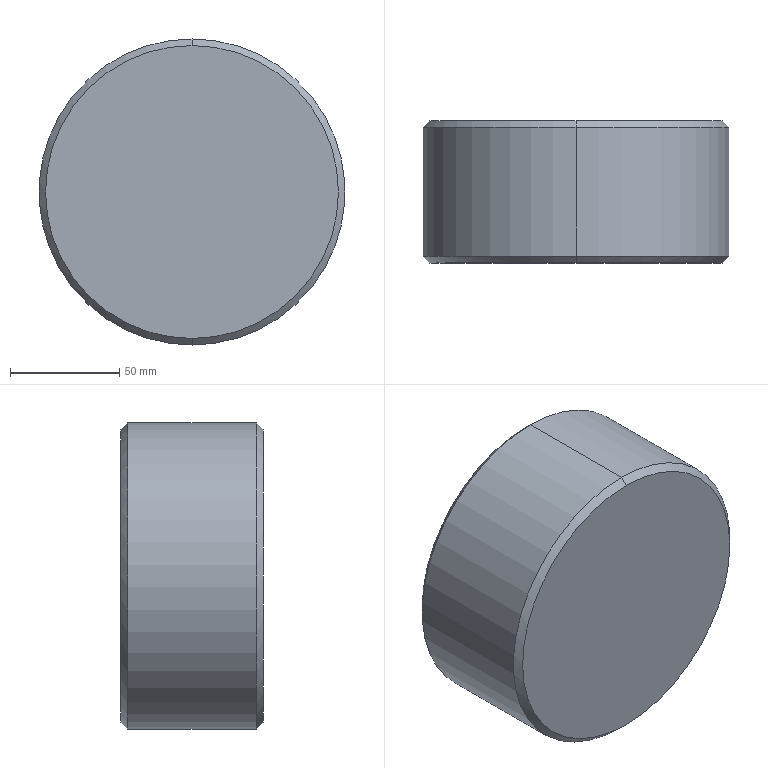Part | SolidWorks | features BaseBody 1 | 1 solid | 13 faces | box 140 x 65 x 140 mm | volume 687379 mm3 | cone 4 | cylinder 4 | plane 3 | sphere 2 | commonest cylinder face diameters 110 x2 140 x2
STEP:
#1=CARTESIAN_POINT('',(234.677,585.635,330.107));
#2=VERTEX_POINT('',#1);
#3=CARTESIAN_POINT('',(234.677,588.635,327.107));
#4=VERTEX_POINT('',#3);
#5=CARTESIAN_POINT('',(234.677,588.635,327.107));
#6=DIRECTION('',(0.,0.7071,-0.7071));
#7=VECTOR('',#6,1000.);
#8=LINE('',#5,#7);
#9=EDGE_CURVE('',#2,#4,#8,.T.);
#10=ORIENTED_EDGE('',*,*,#9,.T.);
#11=CARTESIAN_POINT('',(234.677,588.635,193.107));
#12=VERTEX_POINT('',#11);
#13=CARTESIAN_POINT('',(234.677,588.635,260.107));
#14=DIRECTION('',(0.,1.,0.));
#15=DIRECTION('',(0.,0.,1.));
#16=AXIS2_PLACEMENT_3D('',#13,#14,#15);
#17=CIRCLE('',#16,67.);
#18=EDGE_CURVE('',#12,#4,#17,.T.);
#19=ORIENTED_EDGE('',*,*,#18,.F.);
#20=CARTESIAN_POINT('',(234.677,585.635,190.107));
#21=VERTEX_POINT('',#20);
#22=CARTESIAN_POINT('',(234.677,588.635,193.107));
#23=DIRECTION('',(0.,0.7071,0.7071));
#24=VECTOR('',#23,1000.);
#25=LINE('',#22,#24);
#26=EDGE_CURVE('',#21,#12,#25,.T.);
#27=ORIENTED_EDGE('',*,*,#26,.F.);
#28=CARTESIAN_POINT('',(234.677,585.635,260.107));
#29=DIRECTION('',(0.,-1.,0.));
#30=DIRECTION('',(0.,0.,1.));
#31=AXIS2_PLACEMENT_3D('',#28,#29,#30);
#32=CIRCLE('',#31,70.);
#33=EDGE_CURVE('',#2,#21,#32,.T.);
#34=ORIENTED_EDGE('',*,*,#33,.F.);
#35=EDGE_LOOP('',(#10,#19,#27,#34));
#36=FACE_OUTER_BOUND('',#35,.T.);
#37=CARTESIAN_POINT('',(234.677,588.635,260.107));
#38=DIRECTION('',(0.,-1.,0.));
#39=DIRECTION('',(0.,0.,1.));
#40=AXIS2_PLACEMENT_3D('',#37,#38,#39);
#41=CONICAL_SURFACE('',#40,67.,0.7854);
#42=ADVANCED_FACE('',(#36),#41,.T.);
#43=CARTESIAN_POINT('',(234.677,526.635,190.107));
#44=VERTEX_POINT('',#43);
#45=CARTESIAN_POINT('',(234.677,523.635,193.107));
#46=VERTEX_POINT('',#45);
#47=CARTESIAN_POINT('',(234.677,523.635,193.107));
#48=DIRECTION('',(0.,-0.7071,0.7071));
#49=VECTOR('',#48,1000.);
#50=LINE('',#47,#49);
#51=EDGE_CURVE('',#44,#46,#50,.T.);
#52=ORIENTED_EDGE('',*,*,#51,.T.);
#53=CARTESIAN_POINT('',(234.677,523.635,327.107));
#54=VERTEX_POINT('',#53);
#55=CARTESIAN_POINT('',(234.677,523.635,260.107));
#56=DIRECTION('',(0.,-1.,0.));
#57=DIRECTION('',(0.,0.,1.));
#58=AXIS2_PLACEMENT_3D('',#55,#56,#57);
#59=CIRCLE('',#58,67.);
#60=EDGE_CURVE('',#54,#46,#59,.T.);
#61=ORIENTED_EDGE('',*,*,#60,.F.);
#62=CARTESIAN_POINT('',(234.677,526.635,330.107));
#63=VERTEX_POINT('',#62);
#64=CARTESIAN_POINT('',(234.677,523.635,327.107));
#65=DIRECTION('',(0.,-0.7071,-0.7071));
#66=VECTOR('',#65,1000.);
#67=LINE('',#64,#66);
#68=EDGE_CURVE('',#63,#54,#67,.T.);
#69=ORIENTED_EDGE('',*,*,#68,.F.);
#70=CARTESIAN_POINT('',(234.677,526.635,260.107));
#71=DIRECTION('',(0.,1.,0.));
#72=DIRECTION('',(0.,0.,1.));
#73=AXIS2_PLACEMENT_3D('',#70,#71,#72);
#74=CIRCLE('',#73,70.);
#75=EDGE_CURVE('',#44,#63,#74,.T.);
#76=ORIENTED_EDGE('',*,*,#75,.F.);
#77=EDGE_LOOP('',(#52,#61,#69,#76));
#78=FACE_OUTER_BOUND('',#77,.T.);
#79=CARTESIAN_POINT('',(234.677,523.635,260.107));
#80=DIRECTION('',(0.,1.,0.));
#81=DIRECTION('',(0.,0.,-1.));
#82=AXIS2_PLACEMENT_3D('',#79,#80,#81);
#83=CONICAL_SURFACE('',#82,67.,0.7854);
#84=ADVANCED_FACE('',(#78),#83,.T.);
#85=CARTESIAN_POINT('',(234.677,523.635,330.107));
#86=DIRECTION('',(0.,1.,0.));
#87=VECTOR('',#86,1000.);
#88=LINE('',#85,#87);
#89=EDGE_CURVE('',#63,#2,#88,.T.);
#90=ORIENTED_EDGE('',*,*,#89,.T.);
#91=ORIENTED_EDGE('',*,*,#33,.T.);
#92=CARTESIAN_POINT('',(234.677,523.635,190.107));
#93=DIRECTION('',(0.,1.,0.));
#94=VECTOR('',#93,1000.);
#95=LINE('',#92,#94);
#96=EDGE_CURVE('',#44,#21,#95,.T.);
#97=ORIENTED_EDGE('',*,*,#96,.F.);
#98=ORIENTED_EDGE('',*,*,#75,.T.);
#99=EDGE_LOOP('',(#90,#91,#97,#98));
#100=FACE_OUTER_BOUND('',#99,.T.);
#101=CARTESIAN_POINT('',(234.677,523.635,260.107));
#102=DIRECTION('',(0.,-1.,0.));
#103=DIRECTION('',(0.,0.,1.));
#104=AXIS2_PLACEMENT_3D('',#101,#102,#103);
#105=CYLINDRICAL_SURFACE('',#104,70.);
#106=ADVANCED_FACE('',(#100),#105,.T.);
#107=ORIENTED_EDGE('',*,*,#60,.T.);
#108=CARTESIAN_POINT('',(234.677,523.635,260.107));
#109=DIRECTION('',(0.,-1.,0.));
#110=DIRECTION('',(0.,0.,1.));
#111=AXIS2_PLACEMENT_3D('',#108,#109,#110);
#112=CIRCLE('',#111,67.);
#113=EDGE_CURVE('',#46,#54,#112,.T.);
#114=ORIENTED_EDGE('',*,*,#113,.T.);
#115=EDGE_LOOP('',(#107,#114));
#116=FACE_OUTER_BOUND('',#115,.T.);
#117=CARTESIAN_POINT('',(234.677,523.635,330.107));
#118=DIRECTION('',(0.,1.,0.));
#119=DIRECTION('',(1.,0.,0.));
#120=AXIS2_PLACEMENT_3D('',#117,#118,#119);
#121=PLANE('',#120);
#122=ADVANCED_FACE('',(#116),#121,.F.);
#123=CARTESIAN_POINT('',(234.677,583.635,315.107));
#124=VERTEX_POINT('',#123);
#125=CARTESIAN_POINT('',(234.677,588.635,315.107));
#126=VERTEX_POINT('',#125);
#127=CARTESIAN_POINT('',(234.677,588.635,315.107));
#128=DIRECTION('',(0.,1.,0.));
#129=VECTOR('',#128,1000.);
#130=LINE('',#127,#129);
#131=EDGE_CURVE('',#124,#126,#130,.T.);
#132=ORIENTED_EDGE('',*,*,#131,.T.);
#133=CARTESIAN_POINT('',(234.677,588.635,205.107));
#134=VERTEX_POINT('',#133);
#135=CARTESIAN_POINT('',(234.677,588.635,260.107));
#136=DIRECTION('',(0.,1.,0.));
#137=DIRECTION('',(0.,0.,1.));
#138=AXIS2_PLACEMENT_3D('',#135,#136,#137);
#139=CIRCLE('',#138,55.);
#140=EDGE_CURVE('',#126,#134,#139,.T.);
#141=ORIENTED_EDGE('',*,*,#140,.T.);
#142=CARTESIAN_POINT('',(234.677,583.635,205.107));
#143=VERTEX_POINT('',#142);
#144=CARTESIAN_POINT('',(234.677,588.635,205.107));
#145=DIRECTION('',(0.,1.,0.));
#146=VECTOR('',#145,1000.);
#147=LINE('',#144,#146);
#148=EDGE_CURVE('',#143,#134,#147,.T.);
#149=ORIENTED_EDGE('',*,*,#148,.F.);
#150=CARTESIAN_POINT('',(234.677,583.635,260.107));
#151=DIRECTION('',(0.,1.,0.));
#152=DIRECTION('',(0.,0.,1.));
#153=AXIS2_PLACEMENT_3D('',#150,#151,#152);
#154=CIRCLE('',#153,55.);
#155=EDGE_CURVE('',#124,#143,#154,.T.);
#156=ORIENTED_EDGE('',*,*,#155,.F.);
#157=EDGE_LOOP('',(#132,#141,#149,#156));
#158=FACE_OUTER_BOUND('',#157,.T.);
#159=CARTESIAN_POINT('',(234.677,588.635,260.107));
#160=DIRECTION('',(0.,-1.,0.));
#161=DIRECTION('',(0.,0.,1.));
#162=AXIS2_PLACEMENT_3D('',#159,#160,#161);
#163=CYLINDRICAL_SURFACE('',#162,55.);
#164=ADVANCED_FACE('',(#158),#163,.F.);
#165=CARTESIAN_POINT('',(234.677,588.635,260.107));
#166=DIRECTION('',(0.,1.,0.));
#167=DIRECTION('',(0.,0.,1.));
#168=AXIS2_PLACEMENT_3D('',#165,#166,#167);
#169=CIRCLE('',#168,55.);
#170=EDGE_CURVE('',#134,#126,#169,.T.);
#171=ORIENTED_EDGE('',*,*,#170,.F.);
#172=ORIENTED_EDGE('',*,*,#140,.F.);
#173=EDGE_LOOP('',(#171,#172));
#174=FACE_BOUND('',#173,.T.);
#175=ORIENTED_EDGE('',*,*,#18,.T.);
#176=CARTESIAN_POINT('',(234.677,588.635,260.107));
#177=DIRECTION('',(0.,1.,0.));
#178=DIRECTION('',(0.,0.,1.));
#179=AXIS2_PLACEMENT_3D('',#176,#177,#178);
#180=CIRCLE('',#179,67.);
#181=EDGE_CURVE('',#4,#12,#180,.T.);
#182=ORIENTED_EDGE('',*,*,#181,.T.);
#183=EDGE_LOOP('',(#175,#182));
#184=FACE_OUTER_BOUND('',#183,.T.);
#185=CARTESIAN_POINT('',(234.677,588.635,260.107));
#186=DIRECTION('',(0.,1.,0.));
#187=DIRECTION('',(1.,0.,0.));
#188=AXIS2_PLACEMENT_3D('',#185,#186,#187);
#189=PLANE('',#188);
#190=ADVANCED_FACE('',(#174,#184),#189,.T.);
#191=CARTESIAN_POINT('',(234.677,583.635,210.107));
#192=VERTEX_POINT('',#191);
#193=CARTESIAN_POINT('',(234.677,583.635,310.107));
#194=VERTEX_POINT('',#193);
#195=CARTESIAN_POINT('',(234.677,583.635,260.107));
#196=DIRECTION('',(-1.,0.,0.));
#197=DIRECTION('',(0.,0.,1.));
#198=AXIS2_PLACEMENT_3D('',#195,#196,#197);
#199=CIRCLE('',#198,50.);
#200=EDGE_CURVE('',#192,#194,#199,.T.);
#201=ORIENTED_EDGE('',*,*,#200,.T.);
#202=CARTESIAN_POINT('',(234.677,583.635,260.107));
#203=DIRECTION('',(0.,-1.,0.));
#204=DIRECTION('',(0.,0.,-1.));
#205=AXIS2_PLACEMENT_3D('',#202,#203,#204);
#206=CIRCLE('',#205,50.);
#207=EDGE_CURVE('',#192,#194,#206,.T.);
#208=ORIENTED_EDGE('',*,*,#207,.F.);
#209=EDGE_LOOP('',(#201,#208));
#210=FACE_OUTER_BOUND('',#209,.T.);
#211=CARTESIAN_POINT('',(234.677,583.635,260.107));
#212=DIRECTION('',(-1.,0.,0.));
#213=DIRECTION('',(0.,0.,1.));
#214=AXIS2_PLACEMENT_3D('',#211,#212,#213);
#215=SPHERICAL_SURFACE('',#214,50.);
#216=ADVANCED_FACE('',(#210),#215,.F.);
#217=ORIENTED_EDGE('',*,*,#207,.T.);
#218=CARTESIAN_POINT('',(234.677,583.635,260.107));
#219=DIRECTION('',(0.,-1.,0.));
#220=DIRECTION('',(0.,0.,-1.));
#221=AXIS2_PLACEMENT_3D('',#218,#219,#220);
#222=CIRCLE('',#221,50.);
#223=EDGE_CURVE('',#194,#192,#222,.T.);
#224=ORIENTED_EDGE('',*,*,#223,.T.);
#225=EDGE_LOOP('',(#217,#224));
#226=FACE_BOUND('',#225,.T.);
#227=CARTESIAN_POINT('',(234.677,583.635,260.107));
#228=DIRECTION('',(0.,1.,0.));
#229=DIRECTION('',(0.,0.,1.));
#230=AXIS2_PLACEMENT_3D('',#227,#228,#229);
#231=CIRCLE('',#230,55.);
#232=EDGE_CURVE('',#143,#124,#231,.T.);
#233=ORIENTED_EDGE('',*,*,#232,.T.);
#234=ORIENTED_EDGE('',*,*,#155,.T.);
#235=EDGE_LOOP('',(#233,#234));
#236=FACE_OUTER_BOUND('',#235,.T.);
#237=CARTESIAN_POINT('',(234.677,583.635,330.107));
#238=DIRECTION('',(0.,-1.,0.));
#239=DIRECTION('',(0.,0.,-1.));
#240=AXIS2_PLACEMENT_3D('',#237,#238,#239);
#241=PLANE('',#240);
#242=ADVANCED_FACE('',(#226,#236),#241,.F.);
#243=ORIENTED_EDGE('',*,*,#223,.F.);
#244=ORIENTED_EDGE('',*,*,#200,.F.);
#245=EDGE_LOOP('',(#243,#244));
#246=FACE_OUTER_BOUND('',#245,.T.);
#247=CARTESIAN_POINT('',(234.677,583.635,260.107));
#248=DIRECTION('',(-1.,0.,0.));
#249=DIRECTION('',(0.,0.,1.));
#250=AXIS2_PLACEMENT_3D('',#247,#248,#249);
#251=SPHERICAL_SURFACE('',#250,50.);
#252=ADVANCED_FACE('',(#246),#251,.F.);
#253=ORIENTED_EDGE('',*,*,#170,.T.);
#254=ORIENTED_EDGE('',*,*,#131,.F.);
#255=ORIENTED_EDGE('',*,*,#232,.F.);
#256=ORIENTED_EDGE('',*,*,#148,.T.);
#257=EDGE_LOOP('',(#253,#254,#255,#256));
#258=FACE_OUTER_BOUND('',#257,.T.);
#259=CARTESIAN_POINT('',(234.677,588.635,260.107));
#260=DIRECTION('',(0.,-1.,0.));
#261=DIRECTION('',(0.,0.,1.));
#262=AXIS2_PLACEMENT_3D('',#259,#260,#261);
#263=CYLINDRICAL_SURFACE('',#262,55.);
#264=ADVANCED_FACE('',(#258),#263,.F.);
#265=CARTESIAN_POINT('',(234.677,585.635,260.107));
#266=DIRECTION('',(0.,-1.,0.));
#267=DIRECTION('',(0.,0.,1.));
#268=AXIS2_PLACEMENT_3D('',#265,#266,#267);
#269=CIRCLE('',#268,70.);
#270=EDGE_CURVE('',#21,#2,#269,.T.);
#271=ORIENTED_EDGE('',*,*,#270,.T.);
#272=ORIENTED_EDGE('',*,*,#89,.F.);
#273=CARTESIAN_POINT('',(234.677,526.635,260.107));
#274=DIRECTION('',(0.,1.,0.));
#275=DIRECTION('',(0.,0.,1.));
#276=AXIS2_PLACEMENT_3D('',#273,#274,#275);
#277=CIRCLE('',#276,70.);
#278=EDGE_CURVE('',#63,#44,#277,.T.);
#279=ORIENTED_EDGE('',*,*,#278,.T.);
#280=ORIENTED_EDGE('',*,*,#96,.T.);
#281=EDGE_LOOP('',(#271,#272,#279,#280));
#282=FACE_OUTER_BOUND('',#281,.T.);
#283=CARTESIAN_POINT('',(234.677,523.635,260.107));
#284=DIRECTION('',(0.,-1.,0.));
#285=DIRECTION('',(0.,0.,1.));
#286=AXIS2_PLACEMENT_3D('',#283,#284,#285);
#287=CYLINDRICAL_SURFACE('',#286,70.);
#288=ADVANCED_FACE('',(#282),#287,.T.);
#289=ORIENTED_EDGE('',*,*,#113,.F.);
#290=ORIENTED_EDGE('',*,*,#51,.F.);
#291=ORIENTED_EDGE('',*,*,#278,.F.);
#292=ORIENTED_EDGE('',*,*,#68,.T.);
#293=EDGE_LOOP('',(#289,#290,#291,#292));
#294=FACE_OUTER_BOUND('',#293,.T.);
#295=CARTESIAN_POINT('',(234.677,523.635,260.107));
#296=DIRECTION('',(0.,1.,0.));
#297=DIRECTION('',(0.,0.,-1.));
#298=AXIS2_PLACEMENT_3D('',#295,#296,#297);
#299=CONICAL_SURFACE('',#298,67.,0.7854);
#300=ADVANCED_FACE('',(#294),#299,.T.);
#301=ORIENTED_EDGE('',*,*,#181,.F.);
#302=ORIENTED_EDGE('',*,*,#9,.F.);
#303=ORIENTED_EDGE('',*,*,#270,.F.);
#304=ORIENTED_EDGE('',*,*,#26,.T.);
#305=EDGE_LOOP('',(#301,#302,#303,#304));
#306=FACE_OUTER_BOUND('',#305,.T.);
#307=CARTESIAN_POINT('',(234.677,588.635,260.107));
#308=DIRECTION('',(0.,-1.,0.));
#309=DIRECTION('',(0.,0.,1.));
#310=AXIS2_PLACEMENT_3D('',#307,#308,#309);
#311=CONICAL_SURFACE('',#310,67.,0.7854);
#312=ADVANCED_FACE('',(#306),#311,.T.);
#313=CLOSED_SHELL('',(#42,#84,#106,#122,#164,#190,#216,#242,#252,#264,#288,#300,#312));
#314=MANIFOLD_SOLID_BREP('',#313);
#315=CARTESIAN_POINT('',(0.,0.,0.));
#316=DIRECTION('',(0.,0.,1.));
#317=DIRECTION('',(1.,0.,0.));
#318=AXIS2_PLACEMENT_3D('',#315,#316,#317);
#319=(LENGTH_UNIT()NAMED_UNIT(*)SI_UNIT(.MILLI.,.METRE.));
#320=UNCERTAINTY_MEASURE_WITH_UNIT(LENGTH_MEASURE(0.00001),#319,'','');
#321=(NAMED_UNIT(*)PLANE_ANGLE_UNIT()SI_UNIT($,.RADIAN.));
#322=(NAMED_UNIT(*)SI_UNIT($,.STERADIAN.)SOLID_ANGLE_UNIT());
#323=(GEOMETRIC_REPRESENTATION_CONTEXT(3)GLOBAL_UNCERTAINTY_ASSIGNED_CONTEXT((#320))GLOBAL_UNIT_ASSIGNED_CONTEXT((#319,#321,#322))REPRESENTATION_CONTEXT('',''));
#324=ADVANCED_BREP_SHAPE_REPRESENTATION('',(#314,#318),#323);